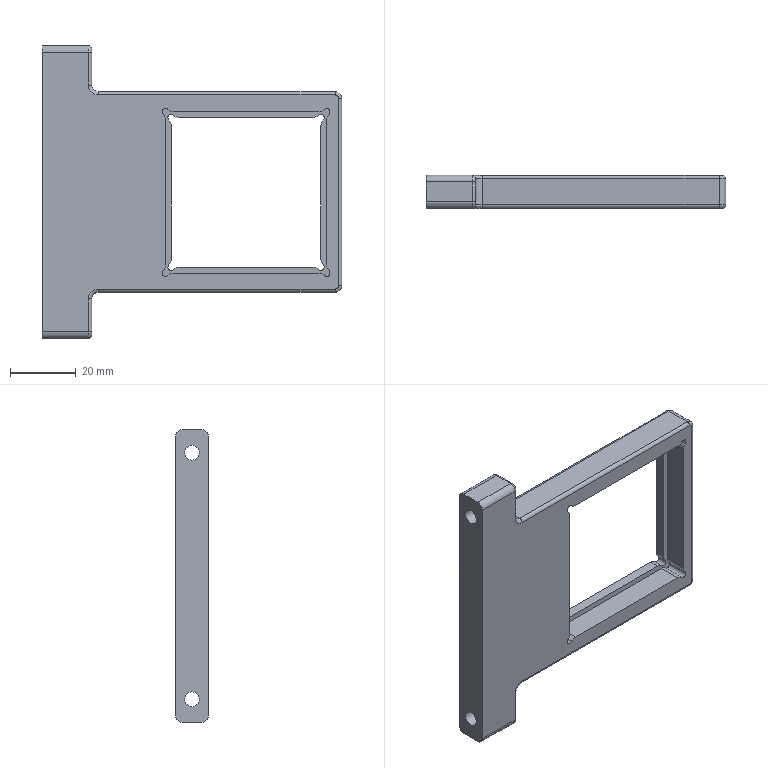NC program | NX | posted by the shop | part box 91 x 10 x 89 mm
Whole program:
%
O0001
(Machine time: 3.69 MIN)
(===Total Tool:3===)
(T1=D80R0.8 face mill D=80.  R=0.8  D-  H01 Z=0.    )
(T19=D4R0.5 D=4.   R=0.5  D-  H19 Z=-2.5  )
(T2=D6 chamfer mill   D=6.   R=0.   D-  H02 Z=-1.2  )
G80 G90 G17 G49 G40
G91 G28 Z0
M01
N1 T01 M06
(D80R0.8 face mill  D=80. R=0.8 H=01 ce=0.10 di=0.10)
G00 G90 G54 X-95.665 Y-23.903 M03 S2800
G43 H01 Z50.
M08
Z3.525
G01 Z1.525 F3000.
X-83.386
X75.619
G02 X81.217 Y-29.503 I-.002 J-5.6
X80.881 Y-31.413 I-5.6 J0.0
G01 X72.51 Y-54.467
G02 X64.991 Y-59.737 I-7.52 J2.73
G01 X-70.597
X-82.597
Z3.525
G00 X-95.665 Y-23.903
Z3.05
G01 Z1.05
X-83.386
X75.619
G02 X81.217 Y-29.503 I-.002 J-5.6
X80.881 Y-31.413 I-5.6 J0.0
G01 X72.51 Y-54.467
G02 X64.991 Y-59.737 I-7.52 J2.73
G01 X-70.597
X-82.597
Z3.05
G00 X-95.665 Y-23.903
Z2.575
G01 Z.575
X-83.386
X75.619
G02 X81.217 Y-29.503 I-.002 J-5.6
X80.881 Y-31.413 I-5.6 J0.0
G01 X72.51 Y-54.467
G02 X64.991 Y-59.737 I-7.52 J2.73
G01 X-70.597
X-82.597
Z2.575
G00 X-95.665 Y-23.903
Z2.1
G01 Z.1
X-83.386
X75.619
G02 X81.217 Y-29.503 I-.002 J-5.6
X80.881 Y-31.413 I-5.6 J0.0
G01 X72.51 Y-54.467
G02 X64.991 Y-59.737 I-7.52 J2.73
G01 X-70.597
X-82.597
Z2.1
G00 Z50.
G91 G28 Z0.0
M05
M09
G91 G28 Z0.0
M01
N2 T01 M06
(D80R0.8 face mill-J  D=80. R=0.8 H=01 ce=0.00 di=0.00)
G00 G90 G54 X-95.547 Y-24.001 M03 S4000
G43 H01 Z50.
M08
Z2.
G01 Z0.0 F1000.
X-83.26
X75.487
G02 X81.085 Y-29.601 I-.002 J-5.6
X80.747 Y-31.516 I-5.6 J0.0
G01 X72.416 Y-54.378
G02 X64.9 Y-59.639 I-7.516 J2.739
G01 X-70.499
X-82.499
Z2.
G00 Z50.
G91 G28 Z0.0
M05
M09
G91 G28 Z0.0
M01
N3 T19 M06
(D4R0.5  D=4. R=0.5 H=19 ce=0.01 di=0.00)
G00 G90 G54 X45.614 Y2.925 M03 S8000
G43 H19 Z11.8
M08
Z.491
G01 Z-.009 F4000.
G03 X44.131 Y1.098 I.515 J-1.933
X44.126 Y.881 I4.112 J-.217
X44.221 Y0.0 I4.118 J0.0
G01 Y-14.
G02 X42.479 Y-15.638 I-1.742 J.107
G01 X42.304 Y-15.63
G03 X41.99 Y-15.614 I-.314 J-3.106
X41.383 Y-15.673 I0.0 J-3.122
G01 Y-15.714 Z-.014
Y-15.747 Z-.019
X42.494 Y-15.707
X42.5 Y-15.726
G03 X44.317 Y-14. I-.028 J1.849
G01 Y0.0
G02 X44.208 Y.815 I2.996 J.815
X44.221 Y1.1 I3.105 J0.0
G01 X44.282 Z-.025
X44.302 Z-.031
G03 X44.287 Y.807 I2.812 J-.293
X44.405 Y0.0 I2.827 J0.0
G01 Y-14.
G02 X42.494 Y-15.794 I-1.919 J.129
G01 X42.212 Y-15.791
X41.402 Y-15.807
X41.383 Y-15.815
Y-15.85 Z-.039
Y-15.881 Z-.047
X42.494 Y-15.877
G03 X44.49 Y-14. I0.0 J1.999
G01 Y0.0
G02 X44.388 Y.804 I3.108 J.804
X44.402 Y1.1 I3.211 J0.0
G01 X44.46 Z-.056
X44.496 Z-.065
G03 X44.483 Y.8 I3.546 J-.3
X44.574 Y0.0 I3.559 J0.0
G01 Y-14.
G02 X42.972 Y-15.876 I-2.026 J.108
X41.972 Y-15.982 I-1. J4.685
X41.383 Y-15.945 I0.0 J4.791
G01 Y-15.979 Z-.075
Y-16.01 Z-.086
G03 X41.928 Y-16.035 I.545 J5.915
X42.932 Y-15.949 I0.0 J5.94
X44.659 Y-14. I-.352 J2.051
G01 Y0.0
G02 X44.554 Y.822 I3.158 J.822
X44.565 Y1.1 I3.263 J0.0
G01 X44.617 Z-.098
X44.645 Z-.11
G03 X44.637 Y.853 I3.457 J-.247
X44.743 Y0.0 I3.465 J0.0
G01 Y-14.
G02 X43.06 Y-16.002 I-2.162 J.109
G01 X42.777 Y-16.031
X42.637 Y-16.068
X41.402
X41.383 Y-16.074
Y-16.106 Z-.124
Y-16.137 Z-.137
X42.641 Y-16.131
X43.024 Y-16.063
G03 X44.828 Y-14. I-.387 J2.158
G01 Y0.0
G02 X44.731 Y.893 I4.079 J.892
X44.736 Y1.1 I4.176 J0.0
G01 X44.781 Z-.152
X44.823 Y1.099 Z-.166
X44.778 Y.674
G02 X44.905 Y0.0 I-2.019 J-.73
G01 Y-14.
G02 X42.67 Y-16.171 I-2.277 J.107
G01 X41.383 Y-16.195
Y-16.228 Z-.183
Y-16.259 Z-.2
X42.777 Y-16.235
X43.06 Y-16.192
G03 X44.99 Y-14. I-.395 J2.294
G01 Y0.0
X44.884 Y.692
X44.897 Y.77
X44.92 Y1.099
X44.967 Z-.219
X45.008 Y1.1 Z-.238
G03 X44.999 Y.815 I4.345 J-.285
X45.076 Y0.0 I4.355 J0.0
G01 Y-14.
G02 X42.977 Y-16.274 I-2.413 J.122
G01 X42.777 Y-16.3
X41.383 Y-16.321
Y-16.353 Z-.259
Y-16.383 Z-.28
G03 X41.918 Y-16.4 I.535 J8.42
X43.06 Y-16.322 I0.0 J8.437
X45.16 Y-14. I-.358 J2.435
G01 Y0.0
G02 X45.076 Y.774 I3.535 J.774
X45.091 Y1.1 I3.618 J0.0
G01 X45.134 Z-.303
X45.175 Z-.326
G03 X45.161 Y.775 I3.655 J-.325
X45.244 Y0.0 I3.67 J0.0
G01 Y-14.
G02 X43.908 Y-16.1 I-2.449 J.084
X42.494 Y-16.441 I-1.438 J2.857
G01 X41.383 Y-16.443
Y-16.473 Z-.35
Y-16.502 Z-.375
X42.494 Y-16.497
G03 X43.908 Y-16.172 I-.009 J3.272
X45.326 Y-14. I-1.077 J2.253
G01 Y0.0
G02 X45.255 Y.788 I4.315 J.788
X45.266 Y1.1 I4.386 J0.0
G01 X45.315 Z-.401
X45.354 Z-.427
G03 X45.341 Y.758 I4.325 J-.341
X45.408 Y0.0 I4.339 J0.0
G01 Y-14.
G02 X44.19 Y-16.091 I-2.521 J.068
X42.494 Y-16.558 I-1.714 J2.911
G01 X41.383
Y-16.586 Z-.455
Y-16.613 Z-.483
X41.402 Y-16.608
X42.494
X42.539
G03 X43.908 Y-16.305 I0.0 J3.238
G01 X44.19 Y-16.167
G03 X45.487 Y-14. I-1.283 J2.24
G01 Y0.0
G02 X45.415 Y.717 I3.544 J.717
X45.435 Y1.099 I3.615 J0.0
G01 X45.476 Z-.513
X45.512 Z-.542
G03 X45.483 Y.754 I2.055 J-.345
X45.501 Y.479 I2.084 J0.0
G01 X45.565 Y0.0
Y-14.
G02 X44.357 Y-16.136 I-2.613 J.068
X42.777 Y-16.646 I-1.772 J2.786
X41.878 Y-16.672 I-.9 J15.592
X41.383 Y-16.664 I0.0 J15.618
G01 Y-16.69 Z-.573
Y-16.713 Z-.604
X42.494 Y-16.711
X42.525 Y-16.712
G03 X44.473 Y-16.137 I0.0 J3.592
X45.64 Y-14. I-1.496 J2.205
G01 Y0.0
G03 X45.594 Y.439 I-3.214 J-.119
G02 X45.563 Y.787 I1.979 J.348
X45.588 Y1.1 I2.009 J0.0
G01 X45.628 Y1.099 Z-.637
X45.667 Z-.67
G03 X45.657 Y.774 I5.337 J-.325
X45.713 Y0.0 I5.347 J0.0
G01 Y-14.
G02 X44.47 Y-16.207 I-2.677 J.054
X42.615 Y-16.752 I-1.876 J2.958
G01 X41.383 Y-16.759
Y-16.781 Z-.704
Y-16.802 Z-.738
X41.402 Y-16.8
X42.494 Y-16.796
X42.715 Y-16.791
G03 X44.48 Y-16.273 I-.079 J3.533
X45.784 Y-14. I-1.423 J2.327
G01 Y0.0
G02 X45.735 Y.726 I5.384 J.726
X45.748 Y1.098 I5.433 J0.0
G01 X45.779 Y1.099 Z-.774
X45.809 Z-.81
G03 X45.799 Y.763 I5.527 J-.336
X45.852 Y0.0 I5.537 J0.0
G01 Y-14.
G02 X44.341 Y-16.419 I-2.801 J.069
G01 X44.19 Y-16.486
G02 X42.777 Y-16.828 I-1.589 J3.474
X41.857 Y-16.847 I-.92 J22.623
X41.383 Y-16.842 I0.0 J22.642
G01 Y-16.86 Z-.847
Y-16.878 Z-.884
X41.402 Y-16.875
X42.494
G03 X43.625 Y-16.736 I-.029 J4.911
X45.038 Y-15.985 I-.777 J3.165
X45.917 Y-14. I-1.903 J2.031
G01 Y0.0
X45.871 Y.459
G02 X45.855 Y.767 I3.019 J.308
X45.873 Y1.1 I3.035 J0.0
G01 X45.906 Z-.922
X45.937 Y1.099 Z-.961
G03 X45.919 Y.766 I3.091 J-.333
X45.934 Y.458 I3.109 J0.0
G01 X45.98 Y0.0
Y-14.
G02 X45.321 Y-15.766 I-2.807 J.042
X43.756 Y-16.741 I-2.357 J2.041
G01 X43.625 Y-16.774
G02 X42.777 Y-16.897 I-1.042 J4.176
X41.929 Y-16.918 I-.848 J17.325
X41.383 Y-16.91 I0.0 J17.346
G01 Y-16.924 Z-1.
Y-16.938 Z-1.04
G03 X41.713 Y-16.939 I.33 J42.027
X42.777 Y-16.926 I0.0 J42.028
X43.759 Y-16.777 I-.081 J3.847
X44.473 Y-16.501 I-.639 J2.716
X46.039 Y-14. I-1.287 J2.547
G01 Y0.0
X45.991 Y.538
G02 X45.984 Y.756 I3.34 J.218
X46.002 Y1.099 I3.347 J0.0
G01 X46.033 Z-1.081
X46.062 Z-1.122
G03 X46.049 Y.723 I5.631 J-.376
X46.096 Y0.0 I5.643 J0.0
G01 Y-14.
G02 X44.755 Y-16.389 I-2.874 J.043
X43.06 Y-16.93 I-1.929 J3.115
X41.96 Y-16.965 I-1.1 J17.421
X41.402 Y-16.956 I0.0 J17.456
G01 X41.383 Y-16.962
Y-16.972 Z-1.164
Y-16.981 Z-1.206
G03 X41.951 Y-16.993 I.568 J13.671
X43.342 Y-16.922 I0.0 J13.683
X44.784 Y-16.419 I-.4 J3.46
X46.149 Y-14. I-1.53 J2.459
G01 Y0.0
X46.106 Y.463
G02 X46.093 Y.74 I2.951 J.277
X46.114 Y1.099 I2.964 J0.0
G01 X46.138 Z-1.249
X46.161 Y1.1 Z-1.292
G03 X46.143 Y.771 I2.952 J-.328
X46.162 Y.429 I2.97 J0.0
G02 X46.199 Y0.0 I-6.942 J-.805
G01 Y-14.
G02 X44.855 Y-16.419 I-2.911 J.035
X43.625 Y-16.9 I-1.789 J2.759
X42.58 Y-16.992 I-1.045 J5.85
G01 X42.494
X41.417
X41.399 Y-16.996
Y-17.005 Z-1.38
X42.777 Y-16.997
X43.06 Y-16.988
G03 X44.388 Y-16.701 I-.159 J3.954
X45.933 Y-15.288 I-1.138 J2.796
X46.245 Y-14. I-2.765 J1.351
G01 Y0.0
X46.205 Y.427
G02 X46.19 Y.761 I3.588 J.334
X46.206 Y1.099 I3.604 J0.0
G01 X46.232 Z-1.425
X46.252 Z-1.47
G03 X46.234 Y.751 I3.372 J-.348
X46.248 Y.444 I3.39 J0.0
G01 X46.288 Y0.0
Y-14.
G02 X45.603 Y-15.864 I-3.014 J.05
X44.19 Y-16.81 I-2.432 J2.105
G01 X43.91 Y-16.883
G02 X43.158 Y-16.992 I-.87 J3.332
G01 X42.777 Y-17.006
X41.408 Y-17.009
Y-17.01 Z-1.562
X42.777
X43.06 Y-17.004
X43.061
G03 X44.473 Y-16.724 I0.0 J3.701
X45.886 Y-15.529 I-1.117 J2.754
G01 X46.007 Y-15.308
X46.024 Y-15.288
G03 X46.327 Y-14. I-2.829 J1.345
G01 Y0.0
G03 X46.295 Y.445 I-6.032 J-.216
G02 X46.278 Y.758 I2.843 J.313
X46.298 Y1.098 I2.86 J0.0
G01 X46.314 Z-1.608
X46.331 Y1.099 Z-1.655
G03 X46.323 Y.753 I7.035 J-.346
X46.363 Y0.0 I7.044 J0.0
G01 Y-14.
G02 X44.473 Y-16.75 I-2.991 J.031
X43.098 Y-17.01 I-1.375 J3.515
G01 X43.06 Y-17.009
X41.408 Y-17.01
Z-1.75
X43.144
G03 X44.183 Y-16.87 I0.0 J3.929
X46.395 Y-14. I-.795 J2.9
G01 Y0.0
X46.362 Y.409
G02 X46.347 Y.766 I4.418 J.357
X46.36 Y1.099 I4.432 J0.0
G01 X46.378 Z-1.798
X46.389 Z-1.846
G03 X46.382 Y.777 I7.402 J-.322
X46.423 Y0.0 I7.409 J0.0
G01 Y-14.
G02 X44.684 Y-16.701 I-3.001 J.022
G01 X44.473 Y-16.793
X44.259 Y-16.86
G02 X43.318 Y-17.008 I-.961 J3.05
G01 X43.06 Y-17.01
X41.408
Z-1.943
X43.342
X43.354
G03 X45.495 Y-16.182 I0.0 J3.182
X46.447 Y-14. I-2.105 J2.218
G01 Y0.0
G02 X46.412 Y.768 I8.37 J.768
X46.418 Y1.1 I8.405 J0.0
G01 X46.432 Z-1.992
X46.448 Z-2.041
G03 X46.442 Y.73 I10.322 J-.37
X46.467 Y0.0 I10.329 J0.0
G01 Y-14.
G02 X45.603 Y-16.1 I-3.077 J.039
X43.394 Y-17.01 I-2.209 J2.225
G01 X43.342
X41.408
Z-2.139
X43.342
X43.376
G03 X44.473 Y-16.831 I0.0 J3.442
X46.484 Y-14. I-1.013 J2.85
G01 Y0.0
G02 X46.464 Y.754 I14.066 J.754
X46.468 Y1.094 I14.086 J0.0
G01 X46.47 Z-2.184
X46.483 Z-2.229
G03 X46.48 Y.77 I19.4 J-.325
X46.495 Y0.0 I19.403 J0.0
G01 Y-14.
G02 X45.906 Y-15.778 I-3.111 J.044
X43.625 Y-17.002 I-2.439 J1.808
G01 X43.342 Y-17.01
X41.408
Z-2.32
X43.342
X43.625 Y-17.004
G03 X46.493 Y-14.158 I-.14 J3.008
G01 X46.498 Y-14.015
X46.503 Y-14.
Y0.0
G02 X46.49 Y.772 I22.338 J.772
X46.492 Y1.094 I22.352 J0.0
G01 X46.502 Z-2.41
X46.508 Y0.0
Y-14.
G02 X43.625 Y-17.006 I-3.019 J.011
G01 X43.342 Y-17.01
X41.408
Z-2.5
X43.342
X43.53 Y-17.008
G03 X46.509 Y-13.999 I-.03 J3.009
G01 X46.51 Y-1.723
Y0.0
Y1.094
G00 Z11.8
X-39.728 Y-17.673
Z.491
G01 Z-.009
Y-17.643
G03 X-41.383 Y-15.673 I-2. J0.0
X-42.035 Y-15.617 I-.652 J-3.728
X-42.352 Y-15.63 I0.0 J-3.785
G01 X-42.497 Y-15.636
G02 X-44.221 Y-14. I0.0 J1.727
G01 Y0.0
X-44.122 Y1.098
X-44.172 Y1.099 Z-.014
X-44.209 Y1.1 Z-.019
G02 X-44.204 Y.898 I-3.622 J-.202
X-44.317 Y0.0 I-3.628 J0.0
G01 Y-14.
G03 X-42.5 Y-15.726 I1.818 J.094
G01 X-42.494 Y-15.707
X-41.383 Y-15.747
Y-15.783 Z-.025
Y-15.815 Z-.031
X-42.643 Y-15.808
X-42.849 Y-15.769
G02 X-44.405 Y-14. I.363 J1.887
G01 Y0.0
G03 X-44.281 Y.9 I-3.203 J.9
X-44.287 Y1.1 I-3.327 J0.0
G01 X-44.352 Z-.039
X-44.381 Z-.047
X-44.49 Y0.0
Y-14.
G03 X-42.777 Y-15.856 I1.991 J.119
G01 X-42.626 Y-15.876
X-41.383 Y-15.881
Y-15.915 Z-.056
Y-15.945 Z-.065
X-41.402 Y-15.944
X-42.522 Y-15.94
G02 X-44.574 Y-14. I.008 J2.065
G01 Y0.0
G03 X-44.478 Y.882 I-3.982 J.882
X-44.484 Y1.1 I-4.079 J0.0
G01 X-44.526 Z-.075
X-44.554 Z-.086
G02 X-44.548 Y.886 I-3.594 J-.214
X-44.659 Y0.0 I-3.6 J0.0
G01 Y-14.
G03 X-42.932 Y-15.949 I2.078 J.102
X-41.928 Y-16.035 I1.004 J5.854
X-41.383 Y-16.01 I0.0 J5.94
G01 Y-16.074 Z-.11
X-41.402 Y-16.068
X-42.637
X-42.777 Y-16.031
X-42.835 Y-16.025
G02 X-44.743 Y-14. I.215 J2.114
G01 Y0.0
G03 X-44.631 Y.912 I-3.654 J.912
G01 X-44.635 Y1.1
X-44.687 Z-.124
X-44.728 Z-.137
X-44.724 Y.913
G02 X-44.828 Y0.0 I-4.061 J0.0
G01 Y-14.
G03 X-42.641 Y-16.131 I2.261 J.133
G01 X-42.494 Y-16.137
X-41.383
Y-16.167 Z-.152
Y-16.195 Z-.166
X-42.67 Y-16.171
G02 X-44.905 Y-14. I.042 J2.279
G01 Y0.0
G03 X-44.809 Y.844 I-3.66 J.844
X-44.817 Y1.099 I-3.756 J0.0
G01 X-44.871 Z-.183
X-44.918 Z-.2
G02 X-44.908 Y.818 I-4.105 J-.281
X-44.99 Y0.0 I-4.115 J0.0
G01 Y-14.
G03 X-43.06 Y-16.192 I2.326 J.102
G01 X-42.777 Y-16.235
X-41.383 Y-16.259
Y-16.291 Z-.219
Y-16.321 Z-.238
X-42.777 Y-16.3
X-42.977 Y-16.274
G02 X-45.076 Y-14. I.314 J2.396
G01 Y0.0
G03 X-44.997 Y.828 I-4.331 J.828
X-45.006 Y1.1 I-4.41 J0.0
G01 X-45.051 Z-.259
X-45.089 Z-.28
G02 X-45.076 Y.782 I-3.65 J-.318
X-45.16 Y0.0 I-3.663 J0.0
G01 Y-14.
G03 X-43.06 Y-16.322 I2.458 J.112
X-41.918 Y-16.4 I1.142 J8.359
X-41.383 Y-16.383 I0.0 J8.437
G01 Y-16.414 Z-.303
Y-16.443 Z-.326
G02 X-41.812 Y-16.449 I-.429 J16.346
X-42.809 Y-16.419 I0.0 J16.352
X-45. Y-15.005 I.182 J2.688
X-45.244 Y-14. I2.869 J1.228
G01 Y0.0
G03 X-45.16 Y.781 I-3.62 J.781
X-45.174 Y1.1 I-3.703 J0.0
G01 X-45.22 Z-.35
X-45.266 Z-.375
G02 X-45.255 Y.792 I-4.406 J-.308
X-45.326 Y0.0 I-4.417 J0.0
G01 Y-14.
X-45.321 Y-14.141
X-45.197 Y-14.723
G03 X-43.06 Y-16.444 I2.487 J.901
X-41.828 Y-16.51 I1.232 J11.373
X-41.383 Y-16.502 I0.0 J11.44
G01 Y-16.531 Z-.401
Y-16.558 Z-.427
X-42.582 Y-16.546
G02 X-44.179 Y-16.098 I.032 J3.179
X-45.408 Y-14. I1.292 J2.166
G01 Y0.0
G03 X-45.341 Y.76 I-4.285 J.76
X-45.354 Y1.1 I-4.352 J0.0
G01 X-45.398 Y1.099 Z-.455
X-45.435 Z-.483
G02 X-45.415 Y.719 I-3.603 J-.38
X-45.487 Y0.0 I-3.623 J0.0
G01 Y-14.
G03 X-45.038 Y-15.397 I2.714 J.102
X-42.958 Y-16.577 I2.389 J1.785
G01 X-42.777 Y-16.596
X-41.383 Y-16.613
Y-16.639 Z-.513
Y-16.664 Z-.542
G02 X-41.908 Y-16.677 I-.525 J10.828
X-42.976 Y-16.624 I0.0 J10.841
X-45.038 Y-15.516 I.3 J3.03
X-45.565 Y-14. I2.196 J1.612
G01 Y0.0
X-45.501 Y.48
G03 X-45.483 Y.754 I-2.062 J.274
X-45.512 Y1.099 I-2.08 J0.0
G01 X-45.55 Z-.573
X-45.587 Y1.1 Z-.604
G02 X-45.563 Y.787 I-1.981 J-.312
X-45.593 Y.439 I-2.005 J0.0
G03 X-45.64 Y0.0 I3.168 J-.558
G01 Y-14.
G03 X-44.473 Y-16.137 I2.664 J.067
X-42.525 Y-16.712 I1.948 J3.017
G01 X-42.494 Y-16.711
X-41.383 Y-16.713
Y-16.737 Z-.637
Y-16.759 Z-.67
X-42.615 Y-16.752
G02 X-44.47 Y-16.207 I.02 J3.503
X-45.713 Y-14. I1.434 J2.261
G01 Y0.0
G03 X-45.657 Y.774 I-5.294 J.774
X-45.667 Y1.099 I-5.351 J0.0
G01 X-45.707 Z-.704
X-45.748 Y1.098 Z-.738
G02 X-45.735 Y.726 I-5.42 J-.372
X-45.784 Y0.0 I-5.433 J0.0
G01 Y-14.
G03 X-44.48 Y-16.273 I2.727 J.054
X-42.715 Y-16.791 I1.843 J3.015
G01 X-42.494 Y-16.796
X-41.402 Y-16.8
X-41.383 Y-16.802
Y-16.823 Z-.774
Y-16.842 Z-.81
G02 X-41.937 Y-16.852 I-.554 J14.549
X-42.777 Y-16.828 I0.0 J14.56
X-44.19 Y-16.486 I.176 J3.816
G01 X-44.341 Y-16.419
G02 X-45.852 Y-14. I1.29 J2.488
G01 Y0.0
G03 X-45.799 Y.763 I-5.482 J.763
X-45.809 Y1.099 I-5.535 J0.0
G01 X-45.844 Z-.847
X-45.873 Y1.1 Z-.884
G02 X-45.855 Y.766 I-2.999 J-.333
X-45.87 Y.46 I-3.017 J0.0
G01 X-45.917 Y0.0
Y-14.
G03 X-45.321 Y-15.676 I2.773 J.043
X-44.19 Y-16.54 I2.326 J1.872
X-43.06 Y-16.841 I1.536 J3.494
X-41.91 Y-16.887 I1.15 J14.257
X-41.383 Y-16.878 I0.0 J14.303
G01 Y-16.894 Z-.922
Y-16.91 Z-.961
G02 X-41.94 Y-16.922 I-.557 J13.01
X-43.06 Y-16.873 I0.0 J13.021
X-44.473 Y-16.452 I.322 J3.657
X-45.886 Y-14.698 I1.373 J2.552
X-45.98 Y-14. I3.86 J.876
G01 Y0.0
X-45.934 Y.459
G03 X-45.919 Y.766 I-3.073 J.306
X-45.937 Y1.099 I-3.088 J0.0
G01 X-45.97 Z-1.
X-46.002 Z-1.04
G02 X-45.984 Y.755 I-3.31 J-.344
X-45.991 Y.538 I-3.328 J0.0
G01 X-46.039 Y0.0
Y-14.
G03 X-45.32 Y-15.853 I2.89 J.055
X-43.908 Y-16.735 I2.311 J2.132
G01 X-43.759 Y-16.777
G03 X-42.777 Y-16.926 I1.063 J3.698
G01 X-41.383 Y-16.938
Y-16.962 Z-1.122
X-41.402 Y-16.956
X-42.494
X-42.56
G02 X-43.763 Y-16.814 I0.0 J5.137
X-45.092 Y-16.136 I.764 J3.142
X-46.096 Y-14. I1.845 J2.17
G01 Y0.0
G03 X-46.049 Y.721 I-5.583 J.721
X-46.062 Y1.099 I-5.629 J0.0
G01 X-46.088 Z-1.164
X-46.115 Z-1.206
G02 X-46.092 Y.739 I-2.877 J-.359
X-46.105 Y.469 I-2.9 J0.0
G01 X-46.149 Y0.0
Y-14.
G03 X-45.038 Y-16.24 I2.891 J.039
X-43.342 Y-16.922 I2.077 J2.713
X-41.951 Y-16.993 I1.391 J13.612
X-41.383 Y-16.981 I0.0 J13.683
G01 X-41.399 Y-16.996 Z-1.292
X-41.417 Y-16.992
X-42.494
X-42.589
G02 X-43.769 Y-16.87 I0.0 J5.735
X-45.505 Y-15.853 I.662 J3.12
X-46.199 Y-14. I2.228 J1.891
G01 Y0.0
G02 X-46.161 Y.441 I6.979 J-.376
G03 X-46.142 Y.769 I-2.792 J.328
X-46.161 Y1.1 I-2.811 J0.0
G01 X-46.185 Y1.099 Z-1.336
X-46.207 Z-1.38
G02 X-46.189 Y.756 I-3.379 J-.344
X-46.204 Y.44 I-3.396 J0.0
G01 X-46.245 Y0.0
Y-14.
G03 X-46.168 Y-14.645 I5.097 J.28
X-44.388 Y-16.701 I2.901 J.713
X-43.06 Y-16.988 I1.487 J3.667
G01 X-42.777 Y-16.997
X-41.399 Y-17.005
X-41.408 Y-17.009 Z-1.47
X-42.777 Y-17.006
X-43.06 Y-16.996
G02 X-44.473 Y-16.697 I.049 J3.72
X-46.192 Y-14.723 I1.167 J2.753
X-46.288 Y-14. I4.317 J.941
G01 Y0.0
X-46.247 Y.446
G03 X-46.233 Y.743 I-3.229 J.298
X-46.253 Y1.099 I-3.243 J0.0
G01 X-46.277 Y1.098 Z-1.516
X-46.3 Z-1.562
G02 X-46.278 Y.749 I-2.747 J-.349
X-46.295 Y.437 I-2.769 J0.0
G03 X-46.327 Y0.0 I5.522 J-.626
G01 Y-14.
G03 X-46.024 Y-15.288 I3.132 J.057
G01 X-46.007 Y-15.308
X-45.886 Y-15.529
G03 X-44.755 Y-16.594 I2.566 J1.59
X-43.06 Y-17.004 I1.696 J3.306
G01 X-42.777 Y-17.01
X-41.399
Z-1.655
X-43.06 Y-17.009
X-43.342 Y-16.999
G02 X-45.321 Y-16.24 I.135 J3.309
X-46.363 Y-14. I1.954 J2.272
G01 Y0.0
X-46.33 Y.416
G03 X-46.318 Y.742 I-4.171 J.326
X-46.333 Y1.098 I-4.184 J0.0
G01 X-46.35 Y1.099 Z-1.702
X-46.363 Z-1.75
G02 X-46.346 Y.758 I-3.387 J-.341
X-46.364 Y.405 I-3.404 J0.0
G03 X-46.395 Y0.0 I7.168 J-.747
G01 Y-14.
G03 X-45.321 Y-16.274 I3.002 J.028
X-43.342 Y-17.004 I2.055 J2.525
G01 X-43.06 Y-17.01
X-41.399
Z-1.846
X-43.06
X-43.342 Y-17.008
G02 X-44.911 Y-16.587 I.059 J3.35
X-46.423 Y-14. I1.499 J2.612
G01 Y0.0
X-46.39 Y.392
G03 X-46.376 Y.727 I-3.958 J.334
X-46.393 Y1.099 I-3.972 J0.0
G01 X-46.412 Z-1.894
X-46.424 Z-1.943
G02 X-46.405 Y.708 I-4.144 J-.392
X-46.417 Y.392 I-4.163 J0.0
G01 X-46.447 Y0.0
Y-14.
G03 X-45.495 Y-16.182 I3.057 J.036
X-43.354 Y-17.01 I2.141 J2.354
G01 X-43.342
X-41.399
Z-2.041
X-43.342
X-43.625 Y-16.998
G02 X-46.172 Y-15.288 I.193 J3.039
X-46.467 Y-14. I2.921 J1.348
G01 Y0.0
X-46.445 Y.372
G03 X-46.436 Y.677 I-5.094 J.305
X-46.453 Y1.094 I-5.103 J0.0
G01 X-46.457 Z-2.09
X-46.471 Z-2.139
G02 X-46.461 Y.663 I-9.763 J-.431
X-46.484 Y0.0 I-9.772 J0.0
G01 Y-14.
G03 X-46.188 Y-15.288 I3.152 J.046
X-43.625 Y-17. I2.731 J1.314
G01 X-43.342 Y-17.01
X-41.399
Z-2.229
X-43.342
X-43.625 Y-17.002
G02 X-46.199 Y-15.288 I.154 J3.02
X-46.495 Y-14. I2.842 J1.333
G01 Y0.0
G03 X-46.479 Y.697 I-14.561 J.697
X-46.484 Y1.094 I-14.578 J0.0
G01 X-46.493 Z-2.32
G02 X-46.489 Y.717 I-18.291 J-.377
X-46.503 Y0.0 I-18.295 J0.0
G01 Y-14.
X-46.498 Y-14.015
G03 X-43.547 Y-17.005 I3.014 J.023
G01 X-43.342 Y-17.01
X-41.399
Z-2.41
X-43.342
X-43.625 Y-17.006
G02 X-46.508 Y-14. I.136 J3.016
G01 Y0.0
X-46.503 Y1.094
X-46.51 Z-2.5
Y0.0
Y-14.007
G03 X-43.54 Y-17.008 I3. J0.0
G01 X-43.342 Y-17.01
X-41.399
G00 Z11.8
G00 G90 X45.57 Y-17.06 M03 S8000
Z11.8
Z.488
G01 Z-.012 F4000.
G03 X43.664 Y-15.663 I-1.907 J-.603
G01 X43.6 Y-15.664
X42.5 Y-15.699
X32.5
G03 X31.199 Y-17. I0.0 J-1.301
G01 Y-89.
G02 X28.5 Y-91.699 I-2.699 J0.0
G01 X-28.5
G02 X-31.199 Y-89. I0.0 J2.699
G01 Y-17.
G03 X-32.5 Y-15.699 I-1.301 J0.0
G01 X-42.5
X-43.6 Y-15.671
Y-15.73 Z-.02
Y-15.78 Z-.029
X-42.5 Y-15.803
X-32.5
G02 X-31.303 Y-17. I0.0 J-1.197
G01 Y-89.
G03 X-28.5 Y-91.803 I2.803 J0.0
G01 X28.5
G03 X31.303 Y-89. I0.0 J2.803
G01 Y-17.
G02 X32.5 Y-15.803 I1.197 J0.0
G01 X42.5
X43.6 Y-15.779
Y-15.838 Z-.041
Y-15.883 Z-.052
X42.5 Y-15.903
X32.5
G03 X31.403 Y-17. I0.0 J-1.097
G01 Y-89.
G02 X28.5 Y-91.903 I-2.903 J0.0
G01 X-28.5
G02 X-31.403 Y-89. I0.0 J2.903
G01 Y-17.
G03 X-32.5 Y-15.903 I-1.097 J0.0
G01 X-42.5
X-43.6 Y-15.881
Y-15.93 Z-.067
Y-15.977 Z-.082
X-42.5 Y-15.998
X-32.5
G02 X-31.498 Y-17. I0.0 J-1.002
G01 Y-89.
G03 X-28.5 Y-91.998 I2.998 J0.0
G01 X28.5
G03 X31.498 Y-89. I0.0 J2.998
G01 Y-17.
G02 X32.5 Y-15.998 I1.002 J0.0
G01 X42.5
X43.6 Y-15.979
Y-16.029 Z-.099
Y-16.06 Z-.117
X42.5 Y-16.091
X32.5
G03 X31.591 Y-17. I0.0 J-.909
G01 Y-89.
G02 X28.5 Y-92.091 I-3.091 J0.0
G01 X-28.5
G02 X-31.591 Y-89. I0.0 J3.091
G01 Y-17.
G03 X-32.5 Y-16.091 I-.909 J0.0
G01 X-42.5
X-43.6 Y-16.059
Y-16.12 Z-.138
Y-16.153 Z-.159
X-42.5 Y-16.182
X-32.5
G02 X-31.682 Y-17. I0.0 J-.818
G01 Y-89.
G03 X-28.5 Y-92.182 I3.182 J0.0
G01 X28.5
G03 X31.682 Y-89. I0.0 J3.182
G01 Y-17.
G02 X32.5 Y-16.182 I.818 J0.0
G01 X42.5
X43.6 Y-16.153
Y-16.212 Z-.183
Y-16.26 Z-.207
X42.5 Y-16.27
X32.5
G03 X31.77 Y-17. I0.0 J-.73
G01 Y-89.
G02 X28.5 Y-92.27 I-3.27 J0.0
G01 X-28.5
G02 X-31.77 Y-89. I0.0 J3.27
G01 Y-17.
G03 X-32.5 Y-16.27 I-.73 J0.0
G01 X-42.5
X-43.6 Y-16.262
Y-16.302 Z-.233
Y-16.335 Z-.26
X-42.5 Y-16.354
X-32.5
G02 X-31.854 Y-17. I0.0 J-.646
G01 Y-89.
G03 X-28.5 Y-92.354 I3.354 J0.0
G01 X28.5
G03 X31.854 Y-89. I0.0 J3.354
G01 Y-17.
G02 X32.5 Y-16.354 I.646 J0.0
G01 X42.5
X43.6 Y-16.34
Y-16.381 Z-.289
Y-16.419 Z-.319
X42.5 Y-16.435
X32.5
G03 X31.935 Y-17. I0.0 J-.565
G01 Y-89.
G02 X28.5 Y-92.435 I-3.435 J0.0
G01 X-28.5
G02 X-31.935 Y-89. I0.0 J3.435
G01 Y-17.
G03 X-32.5 Y-16.435 I-.565 J0.0
G01 X-42.5
X-43.6 Y-16.414
Y-16.454 Z-.351
Y-16.491 Z-.383
X-42.5 Y-16.511
X-32.5
G02 X-32.011 Y-17. I0.0 J-.489
G01 Y-89.
G03 X-28.5 Y-92.511 I3.511 J0.0
G01 X28.5
G03 X32.011 Y-89. I0.0 J3.511
G01 Y-17.
G02 X32.5 Y-16.511 I.489 J0.0
G01 X42.5
X43.6 Y-16.492
Y-16.529 Z-.417
Y-16.568 Z-.452
G03 X43.257 Y-16.564 I-.342 J-14.936
X42.5 Y-16.583 I0.0 J-14.94
G01 X32.5
G03 X32.083 Y-17. I0.0 J-.417
G01 Y-89.
G02 X28.5 Y-92.583 I-3.583 J0.0
G01 X-28.5
G02 X-32.083 Y-89. I0.0 J3.583
G01 Y-17.
G03 X-32.5 Y-16.583 I-.417 J0.0
G01 X-42.5
G03 X-43.264 Y-16.564 I-.764 J-15.487
X-43.6 Y-16.568 I0.0 J-15.506
G01 Y-16.601 Z-.489
Y-16.634 Z-.525
G02 X-43.249 Y-16.629 I.351 J-13.483
X-42.5 Y-16.65 I0.0 J-13.487
G01 X-32.5
G02 X-32.15 Y-17. I0.0 J-.35
G01 Y-89.
G03 X-28.5 Y-92.65 I3.65 J0.0
G01 X28.5
G03 X32.15 Y-89. I0.0 J3.65
G01 Y-17.
G02 X32.5 Y-16.65 I.35 J0.0
G01 X42.5
G02 X43.292 Y-16.63 I.792 J-15.373
X43.6 Y-16.633 I0.0 J-15.394
G01 Y-16.666 Z-.564
X43.601 Y-16.699 Z-.603
X42.5 Y-16.713
X32.5
G03 X32.213 Y-17. I0.0 J-.287
G01 Y-89.
G02 X28.5 Y-92.713 I-3.713 J0.0
G01 X-28.5
G02 X-32.213 Y-89. I0.0 J3.713
G01 Y-17.
G03 X-32.5 Y-16.713 I-.287 J0.0
G01 X-42.5
X-43.553 Y-16.701
X-43.6
Y-16.731 Z-.644
Y-16.764 Z-.685
X-42.5 Y-16.77
X-32.5
G02 X-32.27 Y-17. I0.0 J-.23
G01 Y-89.
G03 X-28.5 Y-92.77 I3.77 J0.0
G01 X28.5
G03 X32.27 Y-89. I0.0 J3.77
G01 Y-17.
G02 X32.5 Y-16.77 I.23 J0.0
G01 X42.5
X43.6 Y-16.762
Y-16.791 Z-.728
Y-16.815 Z-.771
X42.5 Y-16.821
X32.5
G03 X32.321 Y-17. I0.0 J-.179
G01 Y-89.
G02 X28.5 Y-92.821 I-3.821 J0.0
G01 X-28.5
G02 X-32.321 Y-89. I0.0 J3.821
G01 Y-17.
G03 X-32.5 Y-16.821 I-.179 J0.0
G01 X-42.5
X-43.6 Y-16.815
X-43.598 Y-16.838 Z-.816
X-43.597 Y-16.856 Z-.86
G02 X-43.306 Y-16.854 I.291 J-26.192
X-42.5 Y-16.867 I0.0 J-26.194
G01 X-32.5
G02 X-32.367 Y-17. I0.0 J-.133
G01 Y-89.
G03 X-28.5 Y-92.867 I3.867 J0.0
G01 X28.5
G03 X32.367 Y-89. I0.0 J3.867
G01 Y-17.
G02 X32.5 Y-16.867 I.133 J0.0
G01 X42.5
G02 X43.276 Y-16.854 I.776 J-24.303
X43.597 Y-16.857 I0.0 J-24.316
G01 Y-16.878 Z-.906
Y-16.895 Z-.952
G03 X43.269 Y-16.893 I-.328 J-21.707
X42.5 Y-16.906 I0.0 J-21.71
G01 X32.5
X32.448 Y-16.91
X32.41 Y-16.948
X32.406 Y-17.
Y-89.
G02 X28.5 Y-92.906 I-3.906 J0.0
G01 X-28.5
G02 X-32.406 Y-89. I0.0 J3.906
G01 Y-17.
X-32.41 Y-16.948
X-32.448 Y-16.91
X-32.5 Y-16.906
X-42.5
G03 X-43.302 Y-16.893 I-.802 J-24.348
X-43.597 Y-16.895 I0.0 J-24.361
G01 Y-16.914 Z-.999
Y-16.931 Z-1.046
G02 X-43.297 Y-16.929 I.3 J-29.411
X-42.5 Y-16.94 I0.0 J-29.413
G01 X-32.5
X-32.465 Y-16.939
X-32.439 Y-16.965
X-32.44 Y-17.
Y-89.
G03 X-28.5 Y-92.94 I3.94 J0.0
G01 X28.5
G03 X32.44 Y-89. I0.0 J3.94
G01 Y-17.
X32.439 Y-16.965
X32.465 Y-16.939
X32.5 Y-16.94
X42.5
G02 X43.276 Y-16.929 I.776 J-27.033
X43.597 Y-16.931 I0.0 J-27.044
G01 Y-16.942 Z-1.095
Y-16.959 Z-1.143
G03 X42.5 Y-16.967 I.808 J-181.188
G01 X32.5
X32.478 Y-16.963
X32.463 Y-16.978
X32.467 Y-17.
Y-89.
G02 X28.5 Y-92.967 I-3.967 J0.0
G01 X-28.5
G02 X-32.467 Y-89. I0.0 J3.967
G01 Y-17.
X-32.463 Y-16.978
X-32.478 Y-16.963
X-32.5 Y-16.967
X-42.5
G03 X-43.276 Y-16.957 I-.776 J-30.798
X-43.597 Y-16.959 I0.0 J-30.808
G01 Y-16.963 Z-1.187
Y-16.977 Z-1.232
G02 X-43.172 Y-16.971 I.425 J-14.915
X-42.5 Y-16.986 I0.0 J-14.921
G01 X-32.5
X-32.485 Y-16.985
X-32.486 Y-17.
Y-89.
G03 X-28.5 Y-92.986 I3.986 J0.0
G01 X28.5
G03 X32.486 Y-89. I0.0 J3.986
G01 Y-17.
X32.485 Y-16.985
X32.5 Y-16.986
X42.5
G02 X43.262 Y-16.974 I.762 J-25.232
X43.597 Y-16.977 I0.0 J-25.243
G01 Y-16.985 Z-1.277
Y-16.99 Z-1.321
G03 X43.243 Y-16.987 I-.354 J-22.817
X42.5 Y-16.999 I0.0 J-22.82
G01 X32.499
Y-89.
G02 X28.5 Y-92.999 I-3.999 J0.0
G01 X-28.5
G02 X-32.499 Y-89. I0.0 J3.999
G01 Y-16.999
X-42.5
G03 X-43.155 Y-16.982 I-.655 J-12.647
X-43.597 Y-16.99 I0.0 J-12.664
G01 Y-16.994 Z-1.366
Y-17.002 Z-1.411
X-42.5 Y-17.007
X-32.507
Y-89.
G03 X-28.5 Y-93.007 I4.007 J0.0
G01 X28.5
G03 X32.507 Y-89. I0.0 J4.007
G01 Y-17.007
X42.5
X43.597 Y-17.002
Y-17.009 Z-1.5
X32.576 Y-17.01
X32.51
Y-89.
G02 X29.206 Y-92.947 I-4.01 J0.0
X28.5 Y-93.01 I-.705 J3.957
G01 X-28.5
G02 X-32.51 Y-89. I.001 J4.011
G01 Y-17.015
Y-17.01
X-32.515
X-43.597 Y-17.009
G00 Z11.8
G91 G28 Z0.0
M05
M09
G91 G28 Z0.0
M01
N4 T02 M06
(D6 chamfer mill  D=6. R=0. H=02 ce=0.00 di=0.00)
G00 G90 G54 X-42.886 Y1.227 M03 S6500
G43 H02 Z50.
M08
Z.148
G01 Z-1.199 F1500.
G03 X-42.6 Y1.027 I1.286 J1.532
G01 X-42.554 Y.997
X-42.5 Y1.
X42.5
X42.554 Y.997
X42.6 Y1.027
G03 X42.886 Y1.227 I-1. J1.732
G01 Z.148
G00 Z10.
X-.251 Y-83.458
Z.172
G01 Z-1.199
G03 X.035 Y-83.658 I1.286 J1.532
G01 X.08 Y-83.688
X.135 Y-83.685
X20.435
G02 X22.885 Y-84.685 I0.0 J-3.5
X21.885 Y-82.236 I2.5 J2.449
G01 Y-41.635
G02 X22.885 Y-39.185 I3.5 J0.0
X20.435 Y-40.185 I-2.449 J2.5
G01 X-20.166
G02 X-22.615 Y-39.185 I0.0 J3.5
X-21.615 Y-41.635 I-2.5 J-2.449
G01 Y-82.236
G02 X-22.615 Y-84.685 I-3.5 J0.0
X-20.166 Y-83.685 I2.449 J-2.5
G01 X.135
X.189 Y-83.688
X.235 Y-83.658
G03 X.52 Y-83.458 I-1. J1.732
G01 Z.172
G00 Z50.
M05
M09
G91 G28 Z0.0
G91 G28 Y0.0
M30
%